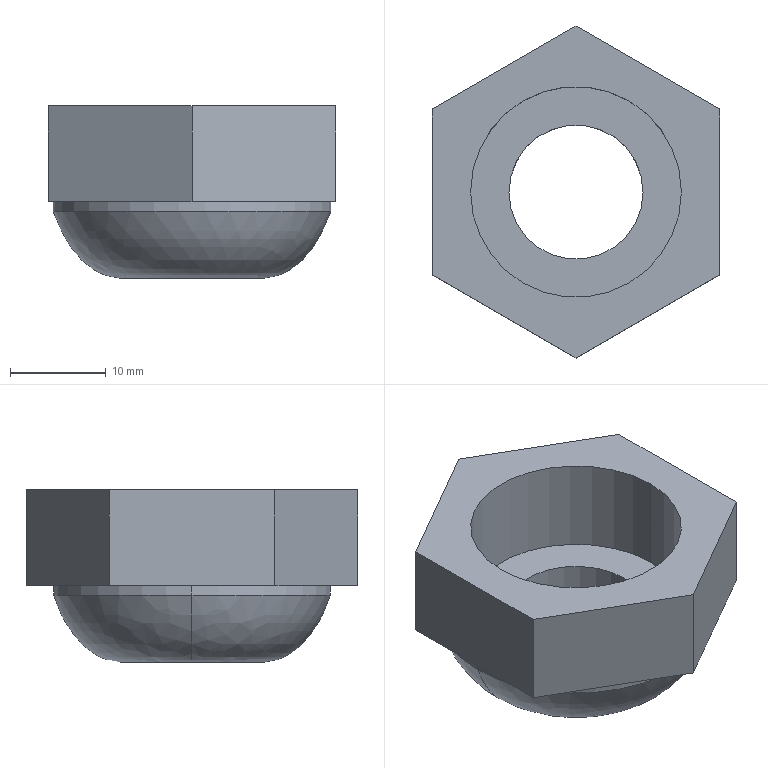Part | NX | features BREP 1 | 1 solid | 18 faces | box 30 x 34.641 x 18 mm | volume 6874 mm3 | plane 10 | cylinder 6 | spline 2 | commonest cylinder face diameters 14 x2 22 x2 29 x2
STEP:
#1=CARTESIAN_POINT('',(-7.5,0.,-8.));
#2=VERTEX_POINT('',#1);
#3=CARTESIAN_POINT('',(7.5,0.,-8.));
#4=VERTEX_POINT('',#3);
#5=CARTESIAN_POINT('',(0.,0.,-8.));
#6=DIRECTION('',(0.,0.,1.));
#7=DIRECTION('',(1.,0.,0.));
#8=AXIS2_PLACEMENT_3D('',#5,#6,#7);
#9=CIRCLE('',#8,7.5);
#10=EDGE_CURVE('',#2,#4,#9,.T.);
#11=ORIENTED_EDGE('',*,*,#10,.T.);
#12=CARTESIAN_POINT('',(14.5,0.,-1.));
#13=VERTEX_POINT('',#12);
#14=CARTESIAN_POINT('',(7.5,0.,-8.));
#15=CARTESIAN_POINT('',(12.09,0.,-7.673));
#16=CARTESIAN_POINT('',(14.5,0.,-1.));
#17=B_SPLINE_CURVE_WITH_KNOTS('',2,(#14,#15,#16),.UNSPECIFIED.,.F.,.F.,(3,3),(0.,1.),.PIECEWISE_BEZIER_KNOTS.);
#18=EDGE_CURVE('',#13,#4,#17,.F.);
#19=ORIENTED_EDGE('',*,*,#18,.F.);
#20=CARTESIAN_POINT('',(-14.5,0.,-1.));
#21=VERTEX_POINT('',#20);
#22=CARTESIAN_POINT('',(0.,0.,-1.));
#23=DIRECTION('',(0.,0.,1.));
#24=DIRECTION('',(1.,0.,0.));
#25=AXIS2_PLACEMENT_3D('',#22,#23,#24);
#26=CIRCLE('',#25,14.5);
#27=EDGE_CURVE('',#21,#13,#26,.T.);
#28=ORIENTED_EDGE('',*,*,#27,.F.);
#29=CARTESIAN_POINT('',(-7.5,0.,-8.));
#30=CARTESIAN_POINT('',(-12.09,0.,-7.673));
#31=CARTESIAN_POINT('',(-14.5,0.,-1.));
#32=B_SPLINE_CURVE_WITH_KNOTS('',2,(#29,#30,#31),.UNSPECIFIED.,.F.,.F.,(3,3),(0.,1.),.PIECEWISE_BEZIER_KNOTS.);
#33=EDGE_CURVE('',#21,#2,#32,.F.);
#34=ORIENTED_EDGE('',*,*,#33,.T.);
#35=EDGE_LOOP('',(#11,#19,#28,#34));
#36=FACE_BOUND('',#35,.T.);
#37=CARTESIAN_POINT('',(-7.5,0.,-8.));
#38=CARTESIAN_POINT('',(-7.5,-15.,-8.));
#39=CARTESIAN_POINT('',(7.5,-15.,-8.));
#40=CARTESIAN_POINT('',(7.5,0.,-8.));
#41=CARTESIAN_POINT('',(-12.09,0.,-7.673));
#42=CARTESIAN_POINT('',(-12.09,-24.179,-7.673));
#43=CARTESIAN_POINT('',(12.09,-24.179,-7.673));
#44=CARTESIAN_POINT('',(12.09,0.,-7.673));
#45=CARTESIAN_POINT('',(-14.5,0.,-1.));
#46=CARTESIAN_POINT('',(-14.5,-29.,-1.));
#47=CARTESIAN_POINT('',(14.5,-29.,-1.));
#48=CARTESIAN_POINT('',(14.5,0.,-1.));
#49=(BOUNDED_SURFACE()B_SPLINE_SURFACE(2,3,((#37,#38,#39,#40),(#41,#42,#43,#44),(#45,#46,#47,#48)),.SURF_OF_REVOLUTION.,.F.,.F.,.F.)B_SPLINE_SURFACE_WITH_KNOTS((3,3),(4,4),(0.,1.),(0.,1.),.PIECEWISE_BEZIER_KNOTS.)GEOMETRIC_REPRESENTATION_ITEM()RATIONAL_B_SPLINE_SURFACE(((1.,0.3333,0.3333,1.),(1.,0.3333,0.3333,1.),(1.,0.3333,0.3333,1.)))REPRESENTATION_ITEM('')SURFACE());
#50=ADVANCED_FACE('',(#36),#49,.F.);
#51=CARTESIAN_POINT('',(-7.,0.,-8.));
#52=VERTEX_POINT('',#51);
#53=CARTESIAN_POINT('',(7.,0.,-8.));
#54=VERTEX_POINT('',#53);
#55=CARTESIAN_POINT('',(0.,0.,-8.));
#56=DIRECTION('',(0.,0.,1.));
#57=DIRECTION('',(1.,0.,0.));
#58=AXIS2_PLACEMENT_3D('',#55,#56,#57);
#59=CIRCLE('',#58,7.);
#60=EDGE_CURVE('',#52,#54,#59,.T.);
#61=ORIENTED_EDGE('',*,*,#60,.F.);
#62=CARTESIAN_POINT('',(-7.,0.,0.));
#63=VERTEX_POINT('',#62);
#64=CARTESIAN_POINT('',(-7.,0.,-8.));
#65=DIRECTION('',(0.,0.,1.));
#66=VECTOR('',#65,1000.);
#67=LINE('',#64,#66);
#68=EDGE_CURVE('',#52,#63,#67,.T.);
#69=ORIENTED_EDGE('',*,*,#68,.T.);
#70=CARTESIAN_POINT('',(7.,0.,0.));
#71=VERTEX_POINT('',#70);
#72=CARTESIAN_POINT('',(0.,0.,0.));
#73=DIRECTION('',(0.,0.,1.));
#74=DIRECTION('',(1.,0.,0.));
#75=AXIS2_PLACEMENT_3D('',#72,#73,#74);
#76=CIRCLE('',#75,7.);
#77=EDGE_CURVE('',#63,#71,#76,.T.);
#78=ORIENTED_EDGE('',*,*,#77,.T.);
#79=CARTESIAN_POINT('',(7.,0.,-8.));
#80=DIRECTION('',(0.,0.,1.));
#81=VECTOR('',#80,1000.);
#82=LINE('',#79,#81);
#83=EDGE_CURVE('',#54,#71,#82,.T.);
#84=ORIENTED_EDGE('',*,*,#83,.F.);
#85=EDGE_LOOP('',(#61,#69,#78,#84));
#86=FACE_BOUND('',#85,.T.);
#87=CARTESIAN_POINT('',(0.,0.,-8.));
#88=DIRECTION('',(0.,0.,1.));
#89=DIRECTION('',(-1.,0.,0.));
#90=AXIS2_PLACEMENT_3D('',#87,#88,#89);
#91=CYLINDRICAL_SURFACE('',#90,7.);
#92=ADVANCED_FACE('',(#86),#91,.F.);
#93=CARTESIAN_POINT('',(0.,0.,-1.));
#94=DIRECTION('',(0.,0.,1.));
#95=DIRECTION('',(1.,0.,0.));
#96=AXIS2_PLACEMENT_3D('',#93,#94,#95);
#97=CIRCLE('',#96,14.5);
#98=EDGE_CURVE('',#13,#21,#97,.T.);
#99=ORIENTED_EDGE('',*,*,#98,.T.);
#100=CARTESIAN_POINT('',(-14.5,0.,0.));
#101=VERTEX_POINT('',#100);
#102=CARTESIAN_POINT('',(-14.5,0.,0.));
#103=DIRECTION('',(0.,0.,1.));
#104=VECTOR('',#103,1000.);
#105=LINE('',#102,#104);
#106=EDGE_CURVE('',#21,#101,#105,.T.);
#107=ORIENTED_EDGE('',*,*,#106,.T.);
#108=CARTESIAN_POINT('',(14.5,0.,0.));
#109=VERTEX_POINT('',#108);
#110=CARTESIAN_POINT('',(0.,0.,0.));
#111=DIRECTION('',(0.,0.,1.));
#112=DIRECTION('',(1.,0.,0.));
#113=AXIS2_PLACEMENT_3D('',#110,#111,#112);
#114=CIRCLE('',#113,14.5);
#115=EDGE_CURVE('',#109,#101,#114,.T.);
#116=ORIENTED_EDGE('',*,*,#115,.F.);
#117=CARTESIAN_POINT('',(14.5,0.,0.));
#118=DIRECTION('',(0.,0.,1.));
#119=VECTOR('',#118,1000.);
#120=LINE('',#117,#119);
#121=EDGE_CURVE('',#13,#109,#120,.T.);
#122=ORIENTED_EDGE('',*,*,#121,.F.);
#123=EDGE_LOOP('',(#99,#107,#116,#122));
#124=FACE_BOUND('',#123,.T.);
#125=CARTESIAN_POINT('',(0.,0.,0.));
#126=DIRECTION('',(0.,0.,1.));
#127=DIRECTION('',(-1.,0.,0.));
#128=AXIS2_PLACEMENT_3D('',#125,#126,#127);
#129=CYLINDRICAL_SURFACE('',#128,14.5);
#130=ADVANCED_FACE('',(#124),#129,.T.);
#131=CARTESIAN_POINT('',(-11.,0.,10.));
#132=VERTEX_POINT('',#131);
#133=CARTESIAN_POINT('',(11.,0.,10.));
#134=VERTEX_POINT('',#133);
#135=CARTESIAN_POINT('',(0.,0.,10.));
#136=DIRECTION('',(0.,0.,1.));
#137=DIRECTION('',(1.,0.,0.));
#138=AXIS2_PLACEMENT_3D('',#135,#136,#137);
#139=CIRCLE('',#138,11.);
#140=EDGE_CURVE('',#132,#134,#139,.T.);
#141=ORIENTED_EDGE('',*,*,#140,.T.);
#142=CARTESIAN_POINT('',(11.,0.,0.));
#143=VERTEX_POINT('',#142);
#144=CARTESIAN_POINT('',(11.,0.,10.));
#145=DIRECTION('',(0.,0.,-1.));
#146=VECTOR('',#145,1000.);
#147=LINE('',#144,#146);
#148=EDGE_CURVE('',#143,#134,#147,.F.);
#149=ORIENTED_EDGE('',*,*,#148,.F.);
#150=CARTESIAN_POINT('',(-11.,0.,0.));
#151=VERTEX_POINT('',#150);
#152=CARTESIAN_POINT('',(0.,0.,0.));
#153=DIRECTION('',(0.,0.,1.));
#154=DIRECTION('',(1.,0.,0.));
#155=AXIS2_PLACEMENT_3D('',#152,#153,#154);
#156=CIRCLE('',#155,11.);
#157=EDGE_CURVE('',#151,#143,#156,.T.);
#158=ORIENTED_EDGE('',*,*,#157,.F.);
#159=CARTESIAN_POINT('',(-11.,0.,10.));
#160=DIRECTION('',(0.,0.,-1.));
#161=VECTOR('',#160,1000.);
#162=LINE('',#159,#161);
#163=EDGE_CURVE('',#151,#132,#162,.F.);
#164=ORIENTED_EDGE('',*,*,#163,.T.);
#165=EDGE_LOOP('',(#141,#149,#158,#164));
#166=FACE_BOUND('',#165,.T.);
#167=CARTESIAN_POINT('',(0.,0.,10.));
#168=DIRECTION('',(0.,0.,-1.));
#169=DIRECTION('',(1.,0.,0.));
#170=AXIS2_PLACEMENT_3D('',#167,#168,#169);
#171=CYLINDRICAL_SURFACE('',#170,11.);
#172=ADVANCED_FACE('',(#166),#171,.F.);
#173=CARTESIAN_POINT('',(15.,8.66,10.));
#174=VERTEX_POINT('',#173);
#175=CARTESIAN_POINT('',(0.,17.321,10.));
#176=VERTEX_POINT('',#175);
#177=CARTESIAN_POINT('',(15.,8.66,10.));
#178=DIRECTION('',(-0.866,0.5,0.));
#179=VECTOR('',#178,1000.);
#180=LINE('',#177,#179);
#181=EDGE_CURVE('',#174,#176,#180,.T.);
#182=ORIENTED_EDGE('',*,*,#181,.T.);
#183=CARTESIAN_POINT('',(-15.,8.66,10.));
#184=VERTEX_POINT('',#183);
#185=CARTESIAN_POINT('',(0.,17.321,10.));
#186=DIRECTION('',(-0.866,-0.5,0.));
#187=VECTOR('',#186,1000.);
#188=LINE('',#185,#187);
#189=EDGE_CURVE('',#176,#184,#188,.T.);
#190=ORIENTED_EDGE('',*,*,#189,.T.);
#191=CARTESIAN_POINT('',(-15.,-8.66,10.));
#192=VERTEX_POINT('',#191);
#193=CARTESIAN_POINT('',(-15.,8.66,10.));
#194=DIRECTION('',(0.,-1.,0.));
#195=VECTOR('',#194,1000.);
#196=LINE('',#193,#195);
#197=EDGE_CURVE('',#184,#192,#196,.T.);
#198=ORIENTED_EDGE('',*,*,#197,.T.);
#199=CARTESIAN_POINT('',(0.,-17.321,10.));
#200=VERTEX_POINT('',#199);
#201=CARTESIAN_POINT('',(-15.,-8.66,10.));
#202=DIRECTION('',(0.866,-0.5,0.));
#203=VECTOR('',#202,1000.);
#204=LINE('',#201,#203);
#205=EDGE_CURVE('',#192,#200,#204,.T.);
#206=ORIENTED_EDGE('',*,*,#205,.T.);
#207=CARTESIAN_POINT('',(15.,-8.66,10.));
#208=VERTEX_POINT('',#207);
#209=CARTESIAN_POINT('',(0.,-17.321,10.));
#210=DIRECTION('',(0.866,0.5,0.));
#211=VECTOR('',#210,1000.);
#212=LINE('',#209,#211);
#213=EDGE_CURVE('',#200,#208,#212,.T.);
#214=ORIENTED_EDGE('',*,*,#213,.T.);
#215=CARTESIAN_POINT('',(15.,-8.66,10.));
#216=DIRECTION('',(0.,1.,0.));
#217=VECTOR('',#216,1000.);
#218=LINE('',#215,#217);
#219=EDGE_CURVE('',#208,#174,#218,.T.);
#220=ORIENTED_EDGE('',*,*,#219,.T.);
#221=EDGE_LOOP('',(#182,#190,#198,#206,#214,#220));
#222=FACE_BOUND('',#221,.T.);
#223=ORIENTED_EDGE('',*,*,#140,.F.);
#224=CARTESIAN_POINT('',(0.,0.,10.));
#225=DIRECTION('',(0.,0.,1.));
#226=DIRECTION('',(1.,0.,0.));
#227=AXIS2_PLACEMENT_3D('',#224,#225,#226);
#228=CIRCLE('',#227,11.);
#229=EDGE_CURVE('',#134,#132,#228,.T.);
#230=ORIENTED_EDGE('',*,*,#229,.F.);
#231=EDGE_LOOP('',(#223,#230));
#232=FACE_BOUND('',#231,.T.);
#233=CARTESIAN_POINT('',(0.,0.,10.));
#234=DIRECTION('',(0.,0.,1.));
#235=DIRECTION('',(-1.,0.,0.));
#236=AXIS2_PLACEMENT_3D('',#233,#234,#235);
#237=PLANE('',#236);
#238=ADVANCED_FACE('',(#222,#232),#237,.T.);
#239=CARTESIAN_POINT('',(15.,8.66,0.));
#240=VERTEX_POINT('',#239);
#241=CARTESIAN_POINT('',(0.,17.321,0.));
#242=VERTEX_POINT('',#241);
#243=CARTESIAN_POINT('',(15.,8.66,0.));
#244=DIRECTION('',(-0.866,0.5,0.));
#245=VECTOR('',#244,1000.);
#246=LINE('',#243,#245);
#247=EDGE_CURVE('',#240,#242,#246,.T.);
#248=ORIENTED_EDGE('',*,*,#247,.F.);
#249=CARTESIAN_POINT('',(15.,-8.66,0.));
#250=VERTEX_POINT('',#249);
#251=CARTESIAN_POINT('',(15.,-8.66,0.));
#252=DIRECTION('',(0.,1.,0.));
#253=VECTOR('',#252,1000.);
#254=LINE('',#251,#253);
#255=EDGE_CURVE('',#250,#240,#254,.T.);
#256=ORIENTED_EDGE('',*,*,#255,.F.);
#257=CARTESIAN_POINT('',(0.,-17.321,0.));
#258=VERTEX_POINT('',#257);
#259=CARTESIAN_POINT('',(0.,-17.321,0.));
#260=DIRECTION('',(0.866,0.5,0.));
#261=VECTOR('',#260,1000.);
#262=LINE('',#259,#261);
#263=EDGE_CURVE('',#258,#250,#262,.T.);
#264=ORIENTED_EDGE('',*,*,#263,.F.);
#265=CARTESIAN_POINT('',(-15.,-8.66,0.));
#266=VERTEX_POINT('',#265);
#267=CARTESIAN_POINT('',(-15.,-8.66,0.));
#268=DIRECTION('',(0.866,-0.5,0.));
#269=VECTOR('',#268,1000.);
#270=LINE('',#267,#269);
#271=EDGE_CURVE('',#266,#258,#270,.T.);
#272=ORIENTED_EDGE('',*,*,#271,.F.);
#273=CARTESIAN_POINT('',(-15.,8.66,0.));
#274=VERTEX_POINT('',#273);
#275=CARTESIAN_POINT('',(-15.,8.66,0.));
#276=DIRECTION('',(0.,-1.,0.));
#277=VECTOR('',#276,1000.);
#278=LINE('',#275,#277);
#279=EDGE_CURVE('',#274,#266,#278,.T.);
#280=ORIENTED_EDGE('',*,*,#279,.F.);
#281=CARTESIAN_POINT('',(0.,17.321,0.));
#282=DIRECTION('',(-0.866,-0.5,0.));
#283=VECTOR('',#282,1000.);
#284=LINE('',#281,#283);
#285=EDGE_CURVE('',#242,#274,#284,.T.);
#286=ORIENTED_EDGE('',*,*,#285,.F.);
#287=EDGE_LOOP('',(#248,#256,#264,#272,#280,#286));
#288=FACE_BOUND('',#287,.T.);
#289=ORIENTED_EDGE('',*,*,#115,.T.);
#290=CARTESIAN_POINT('',(0.,0.,0.));
#291=DIRECTION('',(0.,0.,1.));
#292=DIRECTION('',(1.,0.,0.));
#293=AXIS2_PLACEMENT_3D('',#290,#291,#292);
#294=CIRCLE('',#293,14.5);
#295=EDGE_CURVE('',#101,#109,#294,.T.);
#296=ORIENTED_EDGE('',*,*,#295,.T.);
#297=EDGE_LOOP('',(#289,#296));
#298=FACE_BOUND('',#297,.T.);
#299=CARTESIAN_POINT('',(0.,0.,0.));
#300=DIRECTION('',(0.,0.,1.));
#301=DIRECTION('',(-1.,0.,0.));
#302=AXIS2_PLACEMENT_3D('',#299,#300,#301);
#303=PLANE('',#302);
#304=ADVANCED_FACE('',(#288,#298),#303,.F.);
#305=ORIENTED_EDGE('',*,*,#247,.T.);
#306=CARTESIAN_POINT('',(0.,17.321,10.));
#307=DIRECTION('',(0.,0.,-1.));
#308=VECTOR('',#307,1000.);
#309=LINE('',#306,#308);
#310=EDGE_CURVE('',#176,#242,#309,.T.);
#311=ORIENTED_EDGE('',*,*,#310,.F.);
#312=ORIENTED_EDGE('',*,*,#181,.F.);
#313=CARTESIAN_POINT('',(15.,8.66,10.));
#314=DIRECTION('',(0.,0.,-1.));
#315=VECTOR('',#314,1000.);
#316=LINE('',#313,#315);
#317=EDGE_CURVE('',#174,#240,#316,.T.);
#318=ORIENTED_EDGE('',*,*,#317,.T.);
#319=EDGE_LOOP('',(#305,#311,#312,#318));
#320=FACE_BOUND('',#319,.T.);
#321=CARTESIAN_POINT('',(15.,8.66,10.));
#322=DIRECTION('',(-0.5,-0.866,0.));
#323=DIRECTION('',(0.866,-0.5,0.));
#324=AXIS2_PLACEMENT_3D('',#321,#322,#323);
#325=PLANE('',#324);
#326=ADVANCED_FACE('',(#320),#325,.F.);
#327=ORIENTED_EDGE('',*,*,#285,.T.);
#328=CARTESIAN_POINT('',(-15.,8.66,10.));
#329=DIRECTION('',(0.,0.,-1.));
#330=VECTOR('',#329,1000.);
#331=LINE('',#328,#330);
#332=EDGE_CURVE('',#184,#274,#331,.T.);
#333=ORIENTED_EDGE('',*,*,#332,.F.);
#334=ORIENTED_EDGE('',*,*,#189,.F.);
#335=ORIENTED_EDGE('',*,*,#310,.T.);
#336=EDGE_LOOP('',(#327,#333,#334,#335));
#337=FACE_BOUND('',#336,.T.);
#338=CARTESIAN_POINT('',(0.,17.321,10.));
#339=DIRECTION('',(0.5,-0.866,0.));
#340=DIRECTION('',(0.,0.,1.));
#341=AXIS2_PLACEMENT_3D('',#338,#339,#340);
#342=PLANE('',#341);
#343=ADVANCED_FACE('',(#337),#342,.F.);
#344=ORIENTED_EDGE('',*,*,#279,.T.);
#345=CARTESIAN_POINT('',(-15.,-8.66,10.));
#346=DIRECTION('',(0.,0.,-1.));
#347=VECTOR('',#346,1000.);
#348=LINE('',#345,#347);
#349=EDGE_CURVE('',#192,#266,#348,.T.);
#350=ORIENTED_EDGE('',*,*,#349,.F.);
#351=ORIENTED_EDGE('',*,*,#197,.F.);
#352=ORIENTED_EDGE('',*,*,#332,.T.);
#353=EDGE_LOOP('',(#344,#350,#351,#352));
#354=FACE_BOUND('',#353,.T.);
#355=CARTESIAN_POINT('',(-15.,8.66,10.));
#356=DIRECTION('',(1.,0.,0.));
#357=DIRECTION('',(0.,1.,0.));
#358=AXIS2_PLACEMENT_3D('',#355,#356,#357);
#359=PLANE('',#358);
#360=ADVANCED_FACE('',(#354),#359,.F.);
#361=ORIENTED_EDGE('',*,*,#271,.T.);
#362=CARTESIAN_POINT('',(0.,-17.321,10.));
#363=DIRECTION('',(0.,0.,-1.));
#364=VECTOR('',#363,1000.);
#365=LINE('',#362,#364);
#366=EDGE_CURVE('',#200,#258,#365,.T.);
#367=ORIENTED_EDGE('',*,*,#366,.F.);
#368=ORIENTED_EDGE('',*,*,#205,.F.);
#369=ORIENTED_EDGE('',*,*,#349,.T.);
#370=EDGE_LOOP('',(#361,#367,#368,#369));
#371=FACE_BOUND('',#370,.T.);
#372=CARTESIAN_POINT('',(-15.,-8.66,10.));
#373=DIRECTION('',(0.5,0.866,0.));
#374=DIRECTION('',(0.,0.,1.));
#375=AXIS2_PLACEMENT_3D('',#372,#373,#374);
#376=PLANE('',#375);
#377=ADVANCED_FACE('',(#371),#376,.F.);
#378=ORIENTED_EDGE('',*,*,#263,.T.);
#379=CARTESIAN_POINT('',(15.,-8.66,10.));
#380=DIRECTION('',(0.,0.,-1.));
#381=VECTOR('',#380,1000.);
#382=LINE('',#379,#381);
#383=EDGE_CURVE('',#208,#250,#382,.T.);
#384=ORIENTED_EDGE('',*,*,#383,.F.);
#385=ORIENTED_EDGE('',*,*,#213,.F.);
#386=ORIENTED_EDGE('',*,*,#366,.T.);
#387=EDGE_LOOP('',(#378,#384,#385,#386));
#388=FACE_BOUND('',#387,.T.);
#389=CARTESIAN_POINT('',(0.,-17.321,10.));
#390=DIRECTION('',(-0.5,0.866,0.));
#391=DIRECTION('',(0.,0.,-1.));
#392=AXIS2_PLACEMENT_3D('',#389,#390,#391);
#393=PLANE('',#392);
#394=ADVANCED_FACE('',(#388),#393,.F.);
#395=ORIENTED_EDGE('',*,*,#255,.T.);
#396=ORIENTED_EDGE('',*,*,#317,.F.);
#397=ORIENTED_EDGE('',*,*,#219,.F.);
#398=ORIENTED_EDGE('',*,*,#383,.T.);
#399=EDGE_LOOP('',(#395,#396,#397,#398));
#400=FACE_BOUND('',#399,.T.);
#401=CARTESIAN_POINT('',(15.,-8.66,10.));
#402=DIRECTION('',(-1.,0.,0.));
#403=DIRECTION('',(0.,-1.,0.));
#404=AXIS2_PLACEMENT_3D('',#401,#402,#403);
#405=PLANE('',#404);
#406=ADVANCED_FACE('',(#400),#405,.F.);
#407=ORIENTED_EDGE('',*,*,#148,.T.);
#408=ORIENTED_EDGE('',*,*,#229,.T.);
#409=ORIENTED_EDGE('',*,*,#163,.F.);
#410=CARTESIAN_POINT('',(0.,0.,0.));
#411=DIRECTION('',(0.,0.,1.));
#412=DIRECTION('',(1.,0.,0.));
#413=AXIS2_PLACEMENT_3D('',#410,#411,#412);
#414=CIRCLE('',#413,11.);
#415=EDGE_CURVE('',#143,#151,#414,.T.);
#416=ORIENTED_EDGE('',*,*,#415,.F.);
#417=EDGE_LOOP('',(#407,#408,#409,#416));
#418=FACE_BOUND('',#417,.T.);
#419=CARTESIAN_POINT('',(0.,0.,10.));
#420=DIRECTION('',(0.,0.,-1.));
#421=DIRECTION('',(1.,0.,0.));
#422=AXIS2_PLACEMENT_3D('',#419,#420,#421);
#423=CYLINDRICAL_SURFACE('',#422,11.);
#424=ADVANCED_FACE('',(#418),#423,.F.);
#425=ORIENTED_EDGE('',*,*,#106,.F.);
#426=ORIENTED_EDGE('',*,*,#27,.T.);
#427=ORIENTED_EDGE('',*,*,#121,.T.);
#428=ORIENTED_EDGE('',*,*,#295,.F.);
#429=EDGE_LOOP('',(#425,#426,#427,#428));
#430=FACE_BOUND('',#429,.T.);
#431=CARTESIAN_POINT('',(0.,0.,0.));
#432=DIRECTION('',(0.,0.,1.));
#433=DIRECTION('',(-1.,0.,0.));
#434=AXIS2_PLACEMENT_3D('',#431,#432,#433);
#435=CYLINDRICAL_SURFACE('',#434,14.5);
#436=ADVANCED_FACE('',(#430),#435,.T.);
#437=ORIENTED_EDGE('',*,*,#18,.T.);
#438=CARTESIAN_POINT('',(0.,0.,-8.));
#439=DIRECTION('',(0.,0.,1.));
#440=DIRECTION('',(1.,0.,0.));
#441=AXIS2_PLACEMENT_3D('',#438,#439,#440);
#442=CIRCLE('',#441,7.5);
#443=EDGE_CURVE('',#4,#2,#442,.T.);
#444=ORIENTED_EDGE('',*,*,#443,.T.);
#445=ORIENTED_EDGE('',*,*,#33,.F.);
#446=ORIENTED_EDGE('',*,*,#98,.F.);
#447=EDGE_LOOP('',(#437,#444,#445,#446));
#448=FACE_BOUND('',#447,.T.);
#449=CARTESIAN_POINT('',(7.5,0.,-8.));
#450=CARTESIAN_POINT('',(7.5,15.,-8.));
#451=CARTESIAN_POINT('',(-7.5,15.,-8.));
#452=CARTESIAN_POINT('',(-7.5,0.,-8.));
#453=CARTESIAN_POINT('',(12.09,0.,-7.673));
#454=CARTESIAN_POINT('',(12.09,24.179,-7.673));
#455=CARTESIAN_POINT('',(-12.09,24.179,-7.673));
#456=CARTESIAN_POINT('',(-12.09,0.,-7.673));
#457=CARTESIAN_POINT('',(14.5,0.,-1.));
#458=CARTESIAN_POINT('',(14.5,29.,-1.));
#459=CARTESIAN_POINT('',(-14.5,29.,-1.));
#460=CARTESIAN_POINT('',(-14.5,0.,-1.));
#461=(BOUNDED_SURFACE()B_SPLINE_SURFACE(2,3,((#449,#450,#451,#452),(#453,#454,#455,#456),(#457,#458,#459,#460)),.SURF_OF_REVOLUTION.,.F.,.F.,.F.)B_SPLINE_SURFACE_WITH_KNOTS((3,3),(4,4),(0.,1.),(0.,1.),.PIECEWISE_BEZIER_KNOTS.)GEOMETRIC_REPRESENTATION_ITEM()RATIONAL_B_SPLINE_SURFACE(((1.,0.3333,0.3333,1.),(1.,0.3333,0.3333,1.),(1.,0.3333,0.3333,1.)))REPRESENTATION_ITEM('')SURFACE());
#462=ADVANCED_FACE('',(#448),#461,.F.);
#463=ORIENTED_EDGE('',*,*,#10,.F.);
#464=ORIENTED_EDGE('',*,*,#443,.F.);
#465=EDGE_LOOP('',(#463,#464));
#466=FACE_BOUND('',#465,.T.);
#467=CARTESIAN_POINT('',(0.,0.,-8.));
#468=DIRECTION('',(0.,0.,1.));
#469=DIRECTION('',(1.,0.,0.));
#470=AXIS2_PLACEMENT_3D('',#467,#468,#469);
#471=CIRCLE('',#470,7.);
#472=EDGE_CURVE('',#54,#52,#471,.T.);
#473=ORIENTED_EDGE('',*,*,#472,.T.);
#474=ORIENTED_EDGE('',*,*,#60,.T.);
#475=EDGE_LOOP('',(#473,#474));
#476=FACE_BOUND('',#475,.T.);
#477=CARTESIAN_POINT('',(0.,0.,-8.));
#478=DIRECTION('',(0.,0.,1.));
#479=DIRECTION('',(-1.,0.,0.));
#480=AXIS2_PLACEMENT_3D('',#477,#478,#479);
#481=PLANE('',#480);
#482=ADVANCED_FACE('',(#466,#476),#481,.F.);
#483=ORIENTED_EDGE('',*,*,#157,.T.);
#484=ORIENTED_EDGE('',*,*,#415,.T.);
#485=EDGE_LOOP('',(#483,#484));
#486=FACE_BOUND('',#485,.T.);
#487=CARTESIAN_POINT('',(0.,0.,0.));
#488=DIRECTION('',(0.,0.,1.));
#489=DIRECTION('',(1.,0.,0.));
#490=AXIS2_PLACEMENT_3D('',#487,#488,#489);
#491=CIRCLE('',#490,7.);
#492=EDGE_CURVE('',#71,#63,#491,.T.);
#493=ORIENTED_EDGE('',*,*,#492,.F.);
#494=ORIENTED_EDGE('',*,*,#77,.F.);
#495=EDGE_LOOP('',(#493,#494));
#496=FACE_BOUND('',#495,.T.);
#497=CARTESIAN_POINT('',(-14.5,0.,0.));
#498=DIRECTION('',(0.,0.,-1.));
#499=DIRECTION('',(0.,1.,0.));
#500=AXIS2_PLACEMENT_3D('',#497,#498,#499);
#501=PLANE('',#500);
#502=ADVANCED_FACE('',(#486,#496),#501,.F.);
#503=ORIENTED_EDGE('',*,*,#68,.F.);
#504=ORIENTED_EDGE('',*,*,#472,.F.);
#505=ORIENTED_EDGE('',*,*,#83,.T.);
#506=ORIENTED_EDGE('',*,*,#492,.T.);
#507=EDGE_LOOP('',(#503,#504,#505,#506));
#508=FACE_BOUND('',#507,.T.);
#509=CARTESIAN_POINT('',(0.,0.,-8.));
#510=DIRECTION('',(0.,0.,1.));
#511=DIRECTION('',(-1.,0.,0.));
#512=AXIS2_PLACEMENT_3D('',#509,#510,#511);
#513=CYLINDRICAL_SURFACE('',#512,7.);
#514=ADVANCED_FACE('',(#508),#513,.F.);
#515=CLOSED_SHELL('',(#50,#92,#130,#172,#238,#304,#326,#343,#360,#377,#394,#406,#424,#436,#462,#482,#502,#514));
#516=MANIFOLD_SOLID_BREP('',#515);
#517=(LENGTH_UNIT()NAMED_UNIT(*)SI_UNIT(.MILLI.,.METRE.));
#518=UNCERTAINTY_MEASURE_WITH_UNIT(LENGTH_MEASURE(0.00001),#517,'','');
#519=(NAMED_UNIT(*)PLANE_ANGLE_UNIT()SI_UNIT($,.RADIAN.));
#520=(NAMED_UNIT(*)SI_UNIT($,.STERADIAN.)SOLID_ANGLE_UNIT());
#521=(GEOMETRIC_REPRESENTATION_CONTEXT(3)GLOBAL_UNCERTAINTY_ASSIGNED_CONTEXT((#518))GLOBAL_UNIT_ASSIGNED_CONTEXT((#517,#519,#520))REPRESENTATION_CONTEXT('',''));
#522=ADVANCED_BREP_SHAPE_REPRESENTATION('',(#516),#521);